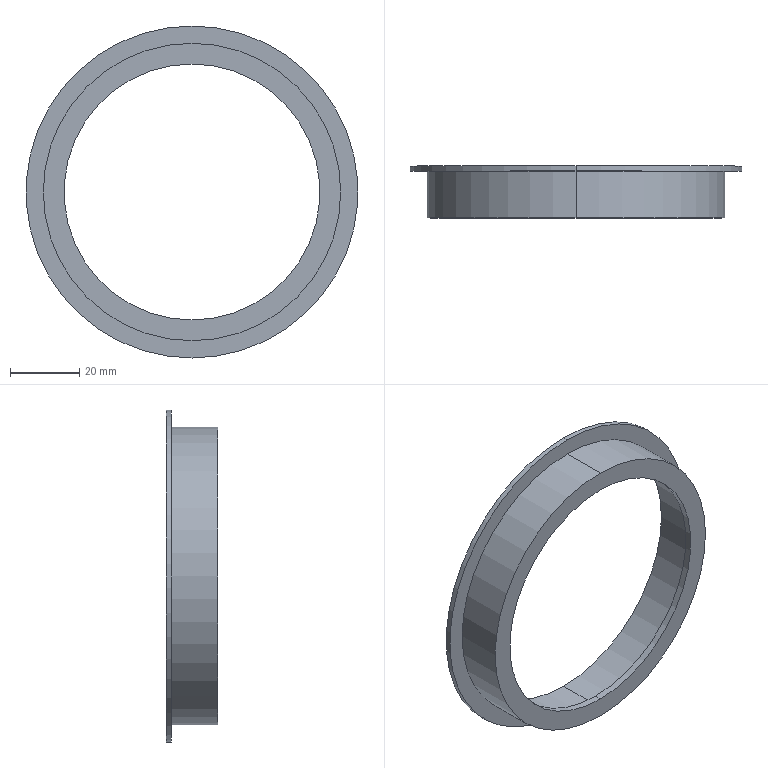Part | SolidWorks | features Revolution 1 | 1 solid | 12 faces | box 96 x 15 x 96 mm | volume 15329 mm3 | cylinder 8 | plane 4 | commonest cylinder face diameters 74 x2 80 x2 86 x2 96 x2
STEP:
#1=CARTESIAN_POINT('',(0.,13.5,-43.));
#2=VERTEX_POINT('',#1);
#3=CARTESIAN_POINT('',(0.,13.5,43.));
#4=VERTEX_POINT('',#3);
#5=CARTESIAN_POINT('',(0.,13.5,0.));
#6=DIRECTION('',(0.,-1.,0.));
#7=DIRECTION('',(0.,0.,-1.));
#8=AXIS2_PLACEMENT_3D('',#5,#6,#7);
#9=CIRCLE('',#8,43.);
#10=EDGE_CURVE('',#2,#4,#9,.T.);
#11=ORIENTED_EDGE('',*,*,#10,.T.);
#12=CARTESIAN_POINT('',(0.,0.,43.));
#13=VERTEX_POINT('',#12);
#14=CARTESIAN_POINT('',(0.,0.,43.));
#15=DIRECTION('',(0.,-1.,0.));
#16=VECTOR('',#15,1000.);
#17=LINE('',#14,#16);
#18=EDGE_CURVE('',#4,#13,#17,.T.);
#19=ORIENTED_EDGE('',*,*,#18,.T.);
#20=CARTESIAN_POINT('',(0.,0.,-43.));
#21=VERTEX_POINT('',#20);
#22=CARTESIAN_POINT('',(0.,0.,0.));
#23=DIRECTION('',(0.,-1.,0.));
#24=DIRECTION('',(0.,0.,-1.));
#25=AXIS2_PLACEMENT_3D('',#22,#23,#24);
#26=CIRCLE('',#25,43.);
#27=EDGE_CURVE('',#21,#13,#26,.T.);
#28=ORIENTED_EDGE('',*,*,#27,.F.);
#29=CARTESIAN_POINT('',(0.,0.,-43.));
#30=DIRECTION('',(0.,-1.,0.));
#31=VECTOR('',#30,1000.);
#32=LINE('',#29,#31);
#33=EDGE_CURVE('',#2,#21,#32,.T.);
#34=ORIENTED_EDGE('',*,*,#33,.F.);
#35=EDGE_LOOP('',(#11,#19,#28,#34));
#36=FACE_OUTER_BOUND('',#35,.T.);
#37=CARTESIAN_POINT('',(0.,0.,0.));
#38=DIRECTION('',(0.,-1.,0.));
#39=DIRECTION('',(0.,0.,-1.));
#40=AXIS2_PLACEMENT_3D('',#37,#38,#39);
#41=CYLINDRICAL_SURFACE('',#40,43.);
#42=ADVANCED_FACE('',(#36),#41,.T.);
#43=CARTESIAN_POINT('',(0.,15.,-48.));
#44=VERTEX_POINT('',#43);
#45=CARTESIAN_POINT('',(0.,15.,48.));
#46=VERTEX_POINT('',#45);
#47=CARTESIAN_POINT('',(0.,15.,0.));
#48=DIRECTION('',(0.,-1.,0.));
#49=DIRECTION('',(0.,0.,-1.));
#50=AXIS2_PLACEMENT_3D('',#47,#48,#49);
#51=CIRCLE('',#50,48.);
#52=EDGE_CURVE('',#44,#46,#51,.T.);
#53=ORIENTED_EDGE('',*,*,#52,.T.);
#54=CARTESIAN_POINT('',(0.,13.5,48.));
#55=VERTEX_POINT('',#54);
#56=CARTESIAN_POINT('',(0.,0.,48.));
#57=DIRECTION('',(0.,-1.,0.));
#58=VECTOR('',#57,1000.);
#59=LINE('',#56,#58);
#60=EDGE_CURVE('',#46,#55,#59,.T.);
#61=ORIENTED_EDGE('',*,*,#60,.T.);
#62=CARTESIAN_POINT('',(0.,13.5,-48.));
#63=VERTEX_POINT('',#62);
#64=CARTESIAN_POINT('',(0.,13.5,0.));
#65=DIRECTION('',(0.,-1.,0.));
#66=DIRECTION('',(0.,0.,-1.));
#67=AXIS2_PLACEMENT_3D('',#64,#65,#66);
#68=CIRCLE('',#67,48.);
#69=EDGE_CURVE('',#63,#55,#68,.T.);
#70=ORIENTED_EDGE('',*,*,#69,.F.);
#71=CARTESIAN_POINT('',(0.,0.,-48.));
#72=DIRECTION('',(0.,-1.,0.));
#73=VECTOR('',#72,1000.);
#74=LINE('',#71,#73);
#75=EDGE_CURVE('',#44,#63,#74,.T.);
#76=ORIENTED_EDGE('',*,*,#75,.F.);
#77=EDGE_LOOP('',(#53,#61,#70,#76));
#78=FACE_OUTER_BOUND('',#77,.T.);
#79=CARTESIAN_POINT('',(0.,0.,0.));
#80=DIRECTION('',(0.,-1.,0.));
#81=DIRECTION('',(0.,0.,-1.));
#82=AXIS2_PLACEMENT_3D('',#79,#80,#81);
#83=CYLINDRICAL_SURFACE('',#82,48.);
#84=ADVANCED_FACE('',(#78),#83,.T.);
#85=CARTESIAN_POINT('',(0.,15.,40.));
#86=VERTEX_POINT('',#85);
#87=CARTESIAN_POINT('',(0.,15.,-40.));
#88=VERTEX_POINT('',#87);
#89=CARTESIAN_POINT('',(0.,15.,0.));
#90=DIRECTION('',(0.,-1.,0.));
#91=DIRECTION('',(0.,0.,-1.));
#92=AXIS2_PLACEMENT_3D('',#89,#90,#91);
#93=CIRCLE('',#92,40.);
#94=EDGE_CURVE('',#86,#88,#93,.T.);
#95=ORIENTED_EDGE('',*,*,#94,.F.);
#96=CARTESIAN_POINT('',(0.,2.,40.));
#97=VERTEX_POINT('',#96);
#98=CARTESIAN_POINT('',(0.,0.,40.));
#99=DIRECTION('',(0.,-1.,0.));
#100=VECTOR('',#99,1000.);
#101=LINE('',#98,#100);
#102=EDGE_CURVE('',#86,#97,#101,.T.);
#103=ORIENTED_EDGE('',*,*,#102,.T.);
#104=CARTESIAN_POINT('',(0.,2.,-40.));
#105=VERTEX_POINT('',#104);
#106=CARTESIAN_POINT('',(0.,2.,0.));
#107=DIRECTION('',(0.,-1.,0.));
#108=DIRECTION('',(0.,0.,-1.));
#109=AXIS2_PLACEMENT_3D('',#106,#107,#108);
#110=CIRCLE('',#109,40.);
#111=EDGE_CURVE('',#97,#105,#110,.T.);
#112=ORIENTED_EDGE('',*,*,#111,.T.);
#113=CARTESIAN_POINT('',(0.,0.,-40.));
#114=DIRECTION('',(0.,-1.,0.));
#115=VECTOR('',#114,1000.);
#116=LINE('',#113,#115);
#117=EDGE_CURVE('',#88,#105,#116,.T.);
#118=ORIENTED_EDGE('',*,*,#117,.F.);
#119=EDGE_LOOP('',(#95,#103,#112,#118));
#120=FACE_OUTER_BOUND('',#119,.T.);
#121=CARTESIAN_POINT('',(0.,0.,0.));
#122=DIRECTION('',(0.,-1.,0.));
#123=DIRECTION('',(0.,0.,-1.));
#124=AXIS2_PLACEMENT_3D('',#121,#122,#123);
#125=CYLINDRICAL_SURFACE('',#124,40.);
#126=ADVANCED_FACE('',(#120),#125,.F.);
#127=CARTESIAN_POINT('',(0.,2.,37.));
#128=VERTEX_POINT('',#127);
#129=CARTESIAN_POINT('',(0.,2.,-37.));
#130=VERTEX_POINT('',#129);
#131=CARTESIAN_POINT('',(0.,2.,0.));
#132=DIRECTION('',(0.,-1.,0.));
#133=DIRECTION('',(0.,0.,-1.));
#134=AXIS2_PLACEMENT_3D('',#131,#132,#133);
#135=CIRCLE('',#134,37.);
#136=EDGE_CURVE('',#128,#130,#135,.T.);
#137=ORIENTED_EDGE('',*,*,#136,.F.);
#138=CARTESIAN_POINT('',(0.,0.,37.));
#139=VERTEX_POINT('',#138);
#140=CARTESIAN_POINT('',(0.,0.,37.));
#141=DIRECTION('',(0.,-1.,0.));
#142=VECTOR('',#141,1000.);
#143=LINE('',#140,#142);
#144=EDGE_CURVE('',#128,#139,#143,.T.);
#145=ORIENTED_EDGE('',*,*,#144,.T.);
#146=CARTESIAN_POINT('',(0.,0.,-37.));
#147=VERTEX_POINT('',#146);
#148=CARTESIAN_POINT('',(0.,0.,0.));
#149=DIRECTION('',(0.,-1.,0.));
#150=DIRECTION('',(0.,0.,-1.));
#151=AXIS2_PLACEMENT_3D('',#148,#149,#150);
#152=CIRCLE('',#151,37.);
#153=EDGE_CURVE('',#139,#147,#152,.T.);
#154=ORIENTED_EDGE('',*,*,#153,.T.);
#155=CARTESIAN_POINT('',(0.,0.,-37.));
#156=DIRECTION('',(0.,-1.,0.));
#157=VECTOR('',#156,1000.);
#158=LINE('',#155,#157);
#159=EDGE_CURVE('',#130,#147,#158,.T.);
#160=ORIENTED_EDGE('',*,*,#159,.F.);
#161=EDGE_LOOP('',(#137,#145,#154,#160));
#162=FACE_OUTER_BOUND('',#161,.T.);
#163=CARTESIAN_POINT('',(0.,0.,0.));
#164=DIRECTION('',(0.,-1.,0.));
#165=DIRECTION('',(0.,0.,-1.));
#166=AXIS2_PLACEMENT_3D('',#163,#164,#165);
#167=CYLINDRICAL_SURFACE('',#166,37.);
#168=ADVANCED_FACE('',(#162),#167,.F.);
#169=CARTESIAN_POINT('',(0.,0.,0.));
#170=DIRECTION('',(0.,-1.,0.));
#171=DIRECTION('',(0.,0.,-1.));
#172=AXIS2_PLACEMENT_3D('',#169,#170,#171);
#173=CIRCLE('',#172,37.);
#174=EDGE_CURVE('',#147,#139,#173,.T.);
#175=ORIENTED_EDGE('',*,*,#174,.F.);
#176=ORIENTED_EDGE('',*,*,#153,.F.);
#177=EDGE_LOOP('',(#175,#176));
#178=FACE_BOUND('',#177,.T.);
#179=ORIENTED_EDGE('',*,*,#27,.T.);
#180=CARTESIAN_POINT('',(0.,0.,0.));
#181=DIRECTION('',(0.,-1.,0.));
#182=DIRECTION('',(0.,0.,-1.));
#183=AXIS2_PLACEMENT_3D('',#180,#181,#182);
#184=CIRCLE('',#183,43.);
#185=EDGE_CURVE('',#13,#21,#184,.T.);
#186=ORIENTED_EDGE('',*,*,#185,.T.);
#187=EDGE_LOOP('',(#179,#186));
#188=FACE_OUTER_BOUND('',#187,.T.);
#189=CARTESIAN_POINT('',(-43.,0.,0.));
#190=DIRECTION('',(0.,1.,0.));
#191=DIRECTION('',(0.,0.,1.));
#192=AXIS2_PLACEMENT_3D('',#189,#190,#191);
#193=PLANE('',#192);
#194=ADVANCED_FACE('',(#178,#188),#193,.F.);
#195=ORIENTED_EDGE('',*,*,#144,.F.);
#196=CARTESIAN_POINT('',(0.,2.,0.));
#197=DIRECTION('',(0.,-1.,0.));
#198=DIRECTION('',(0.,0.,-1.));
#199=AXIS2_PLACEMENT_3D('',#196,#197,#198);
#200=CIRCLE('',#199,37.);
#201=EDGE_CURVE('',#130,#128,#200,.T.);
#202=ORIENTED_EDGE('',*,*,#201,.F.);
#203=ORIENTED_EDGE('',*,*,#159,.T.);
#204=ORIENTED_EDGE('',*,*,#174,.T.);
#205=EDGE_LOOP('',(#195,#202,#203,#204));
#206=FACE_OUTER_BOUND('',#205,.T.);
#207=CARTESIAN_POINT('',(0.,0.,0.));
#208=DIRECTION('',(0.,-1.,0.));
#209=DIRECTION('',(0.,0.,-1.));
#210=AXIS2_PLACEMENT_3D('',#207,#208,#209);
#211=CYLINDRICAL_SURFACE('',#210,37.);
#212=ADVANCED_FACE('',(#206),#211,.F.);
#213=CARTESIAN_POINT('',(0.,2.,0.));
#214=DIRECTION('',(0.,-1.,0.));
#215=DIRECTION('',(0.,0.,-1.));
#216=AXIS2_PLACEMENT_3D('',#213,#214,#215);
#217=CIRCLE('',#216,40.);
#218=EDGE_CURVE('',#105,#97,#217,.T.);
#219=ORIENTED_EDGE('',*,*,#218,.F.);
#220=ORIENTED_EDGE('',*,*,#111,.F.);
#221=EDGE_LOOP('',(#219,#220));
#222=FACE_OUTER_BOUND('',#221,.T.);
#223=ORIENTED_EDGE('',*,*,#201,.T.);
#224=ORIENTED_EDGE('',*,*,#136,.T.);
#225=EDGE_LOOP('',(#223,#224));
#226=FACE_BOUND('',#225,.T.);
#227=CARTESIAN_POINT('',(-37.,2.,0.));
#228=DIRECTION('',(0.,-1.,0.));
#229=DIRECTION('',(0.,0.,-1.));
#230=AXIS2_PLACEMENT_3D('',#227,#228,#229);
#231=PLANE('',#230);
#232=ADVANCED_FACE('',(#222,#226),#231,.F.);
#233=ORIENTED_EDGE('',*,*,#102,.F.);
#234=CARTESIAN_POINT('',(0.,15.,0.));
#235=DIRECTION('',(0.,-1.,0.));
#236=DIRECTION('',(0.,0.,-1.));
#237=AXIS2_PLACEMENT_3D('',#234,#235,#236);
#238=CIRCLE('',#237,40.);
#239=EDGE_CURVE('',#88,#86,#238,.T.);
#240=ORIENTED_EDGE('',*,*,#239,.F.);
#241=ORIENTED_EDGE('',*,*,#117,.T.);
#242=ORIENTED_EDGE('',*,*,#218,.T.);
#243=EDGE_LOOP('',(#233,#240,#241,#242));
#244=FACE_OUTER_BOUND('',#243,.T.);
#245=CARTESIAN_POINT('',(0.,0.,0.));
#246=DIRECTION('',(0.,-1.,0.));
#247=DIRECTION('',(0.,0.,-1.));
#248=AXIS2_PLACEMENT_3D('',#245,#246,#247);
#249=CYLINDRICAL_SURFACE('',#248,40.);
#250=ADVANCED_FACE('',(#244),#249,.F.);
#251=ORIENTED_EDGE('',*,*,#52,.F.);
#252=CARTESIAN_POINT('',(0.,15.,0.));
#253=DIRECTION('',(0.,-1.,0.));
#254=DIRECTION('',(0.,0.,-1.));
#255=AXIS2_PLACEMENT_3D('',#252,#253,#254);
#256=CIRCLE('',#255,48.);
#257=EDGE_CURVE('',#46,#44,#256,.T.);
#258=ORIENTED_EDGE('',*,*,#257,.F.);
#259=EDGE_LOOP('',(#251,#258));
#260=FACE_OUTER_BOUND('',#259,.T.);
#261=ORIENTED_EDGE('',*,*,#239,.T.);
#262=ORIENTED_EDGE('',*,*,#94,.T.);
#263=EDGE_LOOP('',(#261,#262));
#264=FACE_BOUND('',#263,.T.);
#265=CARTESIAN_POINT('',(-40.,15.,0.));
#266=DIRECTION('',(0.,-1.,0.));
#267=DIRECTION('',(0.,0.,-1.));
#268=AXIS2_PLACEMENT_3D('',#265,#266,#267);
#269=PLANE('',#268);
#270=ADVANCED_FACE('',(#260,#264),#269,.F.);
#271=ORIENTED_EDGE('',*,*,#60,.F.);
#272=ORIENTED_EDGE('',*,*,#257,.T.);
#273=ORIENTED_EDGE('',*,*,#75,.T.);
#274=CARTESIAN_POINT('',(0.,13.5,0.));
#275=DIRECTION('',(0.,-1.,0.));
#276=DIRECTION('',(0.,0.,-1.));
#277=AXIS2_PLACEMENT_3D('',#274,#275,#276);
#278=CIRCLE('',#277,48.);
#279=EDGE_CURVE('',#55,#63,#278,.T.);
#280=ORIENTED_EDGE('',*,*,#279,.F.);
#281=EDGE_LOOP('',(#271,#272,#273,#280));
#282=FACE_OUTER_BOUND('',#281,.T.);
#283=CARTESIAN_POINT('',(0.,0.,0.));
#284=DIRECTION('',(0.,-1.,0.));
#285=DIRECTION('',(0.,0.,-1.));
#286=AXIS2_PLACEMENT_3D('',#283,#284,#285);
#287=CYLINDRICAL_SURFACE('',#286,48.);
#288=ADVANCED_FACE('',(#282),#287,.T.);
#289=ORIENTED_EDGE('',*,*,#10,.F.);
#290=CARTESIAN_POINT('',(0.,13.5,0.));
#291=DIRECTION('',(0.,-1.,0.));
#292=DIRECTION('',(0.,0.,-1.));
#293=AXIS2_PLACEMENT_3D('',#290,#291,#292);
#294=CIRCLE('',#293,43.);
#295=EDGE_CURVE('',#4,#2,#294,.T.);
#296=ORIENTED_EDGE('',*,*,#295,.F.);
#297=EDGE_LOOP('',(#289,#296));
#298=FACE_BOUND('',#297,.T.);
#299=ORIENTED_EDGE('',*,*,#69,.T.);
#300=ORIENTED_EDGE('',*,*,#279,.T.);
#301=EDGE_LOOP('',(#299,#300));
#302=FACE_OUTER_BOUND('',#301,.T.);
#303=CARTESIAN_POINT('',(-48.,13.5,0.));
#304=DIRECTION('',(0.,1.,0.));
#305=DIRECTION('',(0.,0.,1.));
#306=AXIS2_PLACEMENT_3D('',#303,#304,#305);
#307=PLANE('',#306);
#308=ADVANCED_FACE('',(#298,#302),#307,.F.);
#309=ORIENTED_EDGE('',*,*,#18,.F.);
#310=ORIENTED_EDGE('',*,*,#295,.T.);
#311=ORIENTED_EDGE('',*,*,#33,.T.);
#312=ORIENTED_EDGE('',*,*,#185,.F.);
#313=EDGE_LOOP('',(#309,#310,#311,#312));
#314=FACE_OUTER_BOUND('',#313,.T.);
#315=CARTESIAN_POINT('',(0.,0.,0.));
#316=DIRECTION('',(0.,-1.,0.));
#317=DIRECTION('',(0.,0.,-1.));
#318=AXIS2_PLACEMENT_3D('',#315,#316,#317);
#319=CYLINDRICAL_SURFACE('',#318,43.);
#320=ADVANCED_FACE('',(#314),#319,.T.);
#321=CLOSED_SHELL('',(#42,#84,#126,#168,#194,#212,#232,#250,#270,#288,#308,#320));
#322=MANIFOLD_SOLID_BREP('',#321);
#323=CARTESIAN_POINT('',(0.,0.,0.));
#324=DIRECTION('',(0.,0.,1.));
#325=DIRECTION('',(1.,0.,0.));
#326=AXIS2_PLACEMENT_3D('',#323,#324,#325);
#327=(LENGTH_UNIT()NAMED_UNIT(*)SI_UNIT(.MILLI.,.METRE.));
#328=UNCERTAINTY_MEASURE_WITH_UNIT(LENGTH_MEASURE(0.00001),#327,'','');
#329=(NAMED_UNIT(*)PLANE_ANGLE_UNIT()SI_UNIT($,.RADIAN.));
#330=(NAMED_UNIT(*)SI_UNIT($,.STERADIAN.)SOLID_ANGLE_UNIT());
#331=(GEOMETRIC_REPRESENTATION_CONTEXT(3)GLOBAL_UNCERTAINTY_ASSIGNED_CONTEXT((#328))GLOBAL_UNIT_ASSIGNED_CONTEXT((#327,#329,#330))REPRESENTATION_CONTEXT('',''));
#332=ADVANCED_BREP_SHAPE_REPRESENTATION('',(#322,#326),#331);